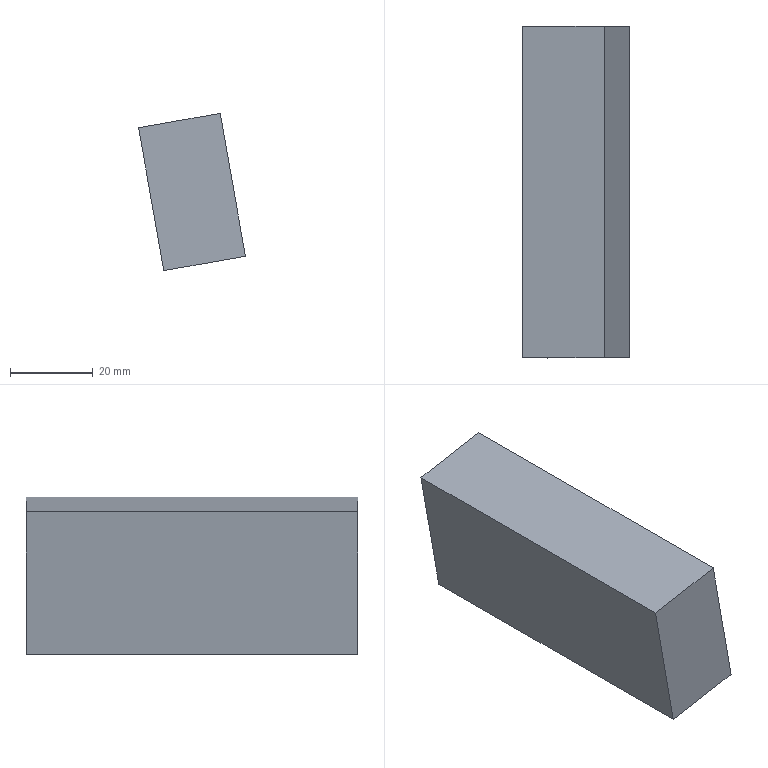Part | NX | features solid 2 | 1 solid | 6 faces | box 25.774 x 80 x 37.941 mm | volume 56000 mm3 | plane 6
STEP:
#1=CARTESIAN_POINT('',(880.991,425.,214.189));
#2=VERTEX_POINT('',#1);
#3=CARTESIAN_POINT('',(880.991,505.,214.189));
#4=VERTEX_POINT('',#3);
#5=CARTESIAN_POINT('',(880.991,465.,214.189));
#6=DIRECTION('',(0.,1.,0.));
#7=VECTOR('',#6,1000.);
#8=LINE('',#5,#7);
#9=EDGE_CURVE('',#2,#4,#8,.T.);
#10=ORIENTED_EDGE('',*,*,#9,.T.);
#11=CARTESIAN_POINT('',(861.295,505.,210.716));
#12=VERTEX_POINT('',#11);
#13=CARTESIAN_POINT('',(861.295,505.,210.716));
#14=DIRECTION('',(0.9848,0.,0.1736));
#15=VECTOR('',#14,1000.);
#16=LINE('',#13,#15);
#17=EDGE_CURVE('',#12,#4,#16,.T.);
#18=ORIENTED_EDGE('',*,*,#17,.F.);
#19=CARTESIAN_POINT('',(861.295,425.,210.716));
#20=VERTEX_POINT('',#19);
#21=CARTESIAN_POINT('',(861.295,465.,210.716));
#22=DIRECTION('',(0.,-1.,0.));
#23=VECTOR('',#22,1000.);
#24=LINE('',#21,#23);
#25=EDGE_CURVE('',#20,#12,#24,.F.);
#26=ORIENTED_EDGE('',*,*,#25,.F.);
#27=CARTESIAN_POINT('',(861.295,425.,210.716));
#28=DIRECTION('',(0.9848,0.,0.1736));
#29=VECTOR('',#28,1000.);
#30=LINE('',#27,#29);
#31=EDGE_CURVE('',#20,#2,#30,.T.);
#32=ORIENTED_EDGE('',*,*,#31,.T.);
#33=EDGE_LOOP('',(#10,#18,#26,#32));
#34=FACE_BOUND('',#33,.T.);
#35=CARTESIAN_POINT('',(861.295,465.,210.716));
#36=DIRECTION('',(0.1736,0.,-0.9848));
#37=DIRECTION('',(0.9848,0.,0.1736));
#38=AXIS2_PLACEMENT_3D('',#35,#36,#37);
#39=PLANE('',#38);
#40=ADVANCED_FACE('',(#34),#39,.F.);
#41=CARTESIAN_POINT('',(887.069,425.,179.721));
#42=VERTEX_POINT('',#41);
#43=CARTESIAN_POINT('',(889.554,425.,165.627));
#44=DIRECTION('',(0.1736,0.,-0.9848));
#45=VECTOR('',#44,1000.);
#46=LINE('',#43,#45);
#47=EDGE_CURVE('',#2,#42,#46,.T.);
#48=ORIENTED_EDGE('',*,*,#47,.F.);
#49=ORIENTED_EDGE('',*,*,#31,.F.);
#50=CARTESIAN_POINT('',(867.373,425.,176.248));
#51=VERTEX_POINT('',#50);
#52=CARTESIAN_POINT('',(869.858,425.,162.154));
#53=DIRECTION('',(0.1736,0.,-0.9848));
#54=VECTOR('',#53,1000.);
#55=LINE('',#52,#54);
#56=EDGE_CURVE('',#20,#51,#55,.T.);
#57=ORIENTED_EDGE('',*,*,#56,.T.);
#58=CARTESIAN_POINT('',(867.373,425.,176.248));
#59=DIRECTION('',(0.9848,0.,0.1736));
#60=VECTOR('',#59,1000.);
#61=LINE('',#58,#60);
#62=EDGE_CURVE('',#51,#42,#61,.T.);
#63=ORIENTED_EDGE('',*,*,#62,.T.);
#64=EDGE_LOOP('',(#48,#49,#57,#63));
#65=FACE_BOUND('',#64,.T.);
#66=CARTESIAN_POINT('',(869.858,425.,162.154));
#67=DIRECTION('',(0.,-1.,0.));
#68=DIRECTION('',(0.,0.,1.));
#69=AXIS2_PLACEMENT_3D('',#66,#67,#68);
#70=PLANE('',#69);
#71=ADVANCED_FACE('',(#65),#70,.T.);
#72=CARTESIAN_POINT('',(887.069,505.,179.721));
#73=VERTEX_POINT('',#72);
#74=CARTESIAN_POINT('',(887.069,465.,179.721));
#75=DIRECTION('',(0.,1.,0.));
#76=VECTOR('',#75,1000.);
#77=LINE('',#74,#76);
#78=EDGE_CURVE('',#42,#73,#77,.T.);
#79=ORIENTED_EDGE('',*,*,#78,.F.);
#80=ORIENTED_EDGE('',*,*,#62,.F.);
#81=CARTESIAN_POINT('',(867.373,505.,176.248));
#82=VERTEX_POINT('',#81);
#83=CARTESIAN_POINT('',(867.373,465.,176.248));
#84=DIRECTION('',(0.,1.,0.));
#85=VECTOR('',#84,1000.);
#86=LINE('',#83,#85);
#87=EDGE_CURVE('',#51,#82,#86,.T.);
#88=ORIENTED_EDGE('',*,*,#87,.T.);
#89=CARTESIAN_POINT('',(867.373,505.,176.248));
#90=DIRECTION('',(0.9848,0.,0.1736));
#91=VECTOR('',#90,1000.);
#92=LINE('',#89,#91);
#93=EDGE_CURVE('',#82,#73,#92,.T.);
#94=ORIENTED_EDGE('',*,*,#93,.T.);
#95=EDGE_LOOP('',(#79,#80,#88,#94));
#96=FACE_BOUND('',#95,.T.);
#97=CARTESIAN_POINT('',(867.373,465.,176.248));
#98=DIRECTION('',(0.1736,0.,-0.9848));
#99=DIRECTION('',(0.9848,0.,0.1736));
#100=AXIS2_PLACEMENT_3D('',#97,#98,#99);
#101=PLANE('',#100);
#102=ADVANCED_FACE('',(#96),#101,.T.);
#103=CARTESIAN_POINT('',(875.502,505.,245.321));
#104=DIRECTION('',(0.1736,0.,-0.9848));
#105=VECTOR('',#104,1000.);
#106=LINE('',#103,#105);
#107=EDGE_CURVE('',#4,#73,#106,.T.);
#108=ORIENTED_EDGE('',*,*,#107,.T.);
#109=ORIENTED_EDGE('',*,*,#93,.F.);
#110=CARTESIAN_POINT('',(855.806,505.,241.848));
#111=DIRECTION('',(0.1736,0.,-0.9848));
#112=VECTOR('',#111,1000.);
#113=LINE('',#110,#112);
#114=EDGE_CURVE('',#12,#82,#113,.T.);
#115=ORIENTED_EDGE('',*,*,#114,.F.);
#116=ORIENTED_EDGE('',*,*,#17,.T.);
#117=EDGE_LOOP('',(#108,#109,#115,#116));
#118=FACE_BOUND('',#117,.T.);
#119=CARTESIAN_POINT('',(855.806,505.,241.848));
#120=DIRECTION('',(0.,-1.,0.));
#121=DIRECTION('',(0.,0.,1.));
#122=AXIS2_PLACEMENT_3D('',#119,#120,#121);
#123=PLANE('',#122);
#124=ADVANCED_FACE('',(#118),#123,.F.);
#125=ORIENTED_EDGE('',*,*,#25,.T.);
#126=ORIENTED_EDGE('',*,*,#114,.T.);
#127=ORIENTED_EDGE('',*,*,#87,.F.);
#128=ORIENTED_EDGE('',*,*,#56,.F.);
#129=EDGE_LOOP('',(#125,#126,#127,#128));
#130=FACE_BOUND('',#129,.T.);
#131=CARTESIAN_POINT('',(855.806,465.,241.848));
#132=DIRECTION('',(-0.9848,0.,-0.1736));
#133=DIRECTION('',(0.1736,0.,-0.9848));
#134=AXIS2_PLACEMENT_3D('',#131,#132,#133);
#135=PLANE('',#134);
#136=ADVANCED_FACE('',(#130),#135,.T.);
#137=ORIENTED_EDGE('',*,*,#9,.F.);
#138=ORIENTED_EDGE('',*,*,#47,.T.);
#139=ORIENTED_EDGE('',*,*,#78,.T.);
#140=ORIENTED_EDGE('',*,*,#107,.F.);
#141=EDGE_LOOP('',(#137,#138,#139,#140));
#142=FACE_BOUND('',#141,.T.);
#143=CARTESIAN_POINT('',(875.502,465.,245.321));
#144=DIRECTION('',(-0.9848,0.,-0.1736));
#145=DIRECTION('',(0.1736,0.,-0.9848));
#146=AXIS2_PLACEMENT_3D('',#143,#144,#145);
#147=PLANE('',#146);
#148=ADVANCED_FACE('',(#142),#147,.F.);
#149=CLOSED_SHELL('',(#40,#71,#102,#124,#136,#148));
#150=MANIFOLD_SOLID_BREP('',#149);
#151=(LENGTH_UNIT()NAMED_UNIT(*)SI_UNIT(.MILLI.,.METRE.));
#152=UNCERTAINTY_MEASURE_WITH_UNIT(LENGTH_MEASURE(0.00001),#151,'','');
#153=(NAMED_UNIT(*)PLANE_ANGLE_UNIT()SI_UNIT($,.RADIAN.));
#154=(NAMED_UNIT(*)SI_UNIT($,.STERADIAN.)SOLID_ANGLE_UNIT());
#155=(GEOMETRIC_REPRESENTATION_CONTEXT(3)GLOBAL_UNCERTAINTY_ASSIGNED_CONTEXT((#152))GLOBAL_UNIT_ASSIGNED_CONTEXT((#151,#153,#154))REPRESENTATION_CONTEXT('',''));
#156=ADVANCED_BREP_SHAPE_REPRESENTATION('',(#150),#155);